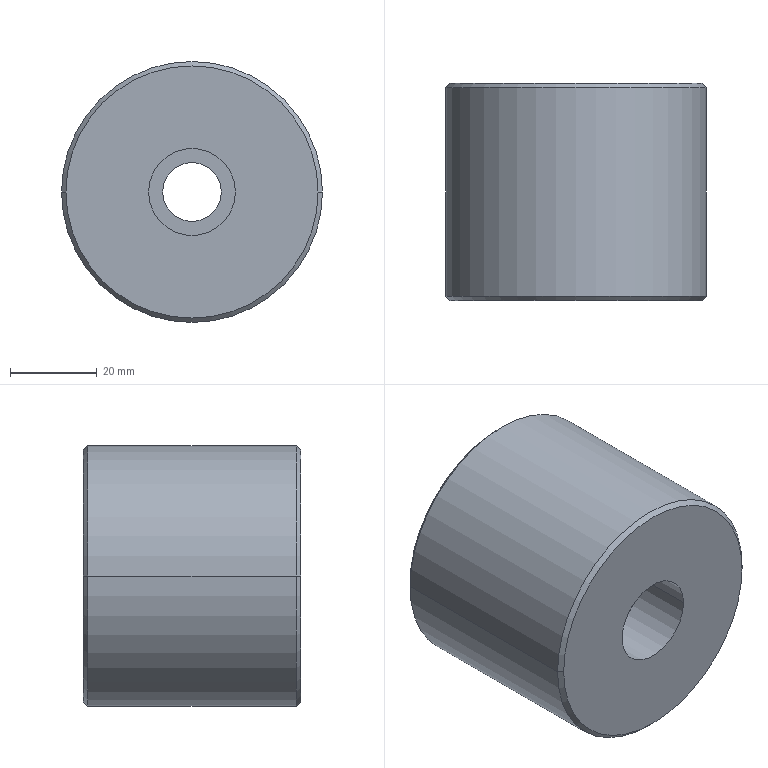Part | Creo | 1 solid | 13 faces | box 60 x 50 x 60 mm | volume 131634 mm3 | cylinder 6 | cone 4 | plane 3 | commonest cylinder face diameters 13.5 x2 20 x2 60 x2
STEP:
#1=CARTESIAN_POINT('',(0.,0.,0.));
#2=DIRECTION('',(0.,0.,1.));
#3=DIRECTION('',(1.,0.,0.));
#4=AXIS2_PLACEMENT_3D('',#1,#2,#3);
#5=CARTESIAN_POINT('',(-195.,-251.,-52.5));
#6=VERTEX_POINT('',#5);
#7=CARTESIAN_POINT('',(-135.,-251.,-52.5));
#8=VERTEX_POINT('',#7);
#9=CARTESIAN_POINT('',(-165.,-251.,-52.5));
#10=DIRECTION('',(0.,1.,0.));
#11=DIRECTION('',(-1.,0.,0.));
#12=AXIS2_PLACEMENT_3D('',#9,#10,#11);
#13=CIRCLE('',#12,30.);
#14=EDGE_CURVE('',#6,#8,#13,.T.);
#15=ORIENTED_EDGE('',*,*,#14,.T.);
#16=CARTESIAN_POINT('',(-135.,-299.,-52.5));
#17=VERTEX_POINT('',#16);
#18=CARTESIAN_POINT('',(-135.,-299.,-52.5));
#19=DIRECTION('',(0.,1.,0.));
#20=VECTOR('',#19,48.);
#21=LINE('',#18,#20);
#22=EDGE_CURVE('',#17,#8,#21,.T.);
#23=ORIENTED_EDGE('',*,*,#22,.F.);
#24=CARTESIAN_POINT('',(-195.,-299.,-52.5));
#25=VERTEX_POINT('',#24);
#26=CARTESIAN_POINT('',(-165.,-299.,-52.5));
#27=DIRECTION('',(0.,-1.,0.));
#28=DIRECTION('',(1.,0.,0.));
#29=AXIS2_PLACEMENT_3D('',#26,#27,#28);
#30=CIRCLE('',#29,30.);
#31=EDGE_CURVE('',#17,#25,#30,.T.);
#32=ORIENTED_EDGE('',*,*,#31,.T.);
#33=CARTESIAN_POINT('',(-195.,-299.,-52.5));
#34=DIRECTION('',(0.,1.,0.));
#35=VECTOR('',#34,48.);
#36=LINE('',#33,#35);
#37=EDGE_CURVE('',#25,#6,#36,.T.);
#38=ORIENTED_EDGE('',*,*,#37,.T.);
#39=EDGE_LOOP('',(#15,#23,#32,#38));
#40=FACE_OUTER_BOUND('',#39,.F.);
#41=CARTESIAN_POINT('',(-165.,-300.,-52.5));
#42=DIRECTION('',(0.,1.,0.));
#43=DIRECTION('',(-1.,0.,0.));
#44=AXIS2_PLACEMENT_3D('',#41,#42,#43);
#45=CYLINDRICAL_SURFACE('',#44,30.);
#46=ADVANCED_FACE('',(#40),#45,.T.);
#47=CARTESIAN_POINT('',(-194.,-250.,-52.5));
#48=VERTEX_POINT('',#47);
#49=CARTESIAN_POINT('',(-136.,-250.,-52.5));
#50=VERTEX_POINT('',#49);
#51=CARTESIAN_POINT('',(-165.,-250.,-52.5));
#52=DIRECTION('',(0.,1.,0.));
#53=DIRECTION('',(-1.,0.,0.));
#54=AXIS2_PLACEMENT_3D('',#51,#52,#53);
#55=CIRCLE('',#54,29.);
#56=EDGE_CURVE('',#48,#50,#55,.T.);
#57=ORIENTED_EDGE('',*,*,#56,.T.);
#58=CARTESIAN_POINT('',(-136.,-250.,-52.5));
#59=DIRECTION('',(0.7071,-0.7071,0.));
#60=VECTOR('',#59,1.414);
#61=LINE('',#58,#60);
#62=EDGE_CURVE('',#50,#8,#61,.T.);
#63=ORIENTED_EDGE('',*,*,#62,.T.);
#64=ORIENTED_EDGE('',*,*,#14,.F.);
#65=CARTESIAN_POINT('',(-194.,-250.,-52.5));
#66=DIRECTION('',(-0.7071,-0.7071,0.));
#67=VECTOR('',#66,1.414);
#68=LINE('',#65,#67);
#69=EDGE_CURVE('',#48,#6,#68,.T.);
#70=ORIENTED_EDGE('',*,*,#69,.F.);
#71=EDGE_LOOP('',(#57,#63,#64,#70));
#72=FACE_OUTER_BOUND('',#71,.F.);
#73=CARTESIAN_POINT('',(-165.,-250.5,-52.5));
#74=DIRECTION('',(0.,-1.,0.));
#75=DIRECTION('',(1.,0.,0.));
#76=AXIS2_PLACEMENT_3D('',#73,#74,#75);
#77=CONICAL_SURFACE('',#76,29.5,45.);
#78=ADVANCED_FACE('',(#72),#77,.T.);
#79=CARTESIAN_POINT('',(-165.,-250.,-52.5));
#80=DIRECTION('',(0.,1.,0.));
#81=DIRECTION('',(1.,0.,0.));
#82=AXIS2_PLACEMENT_3D('',#79,#80,#81);
#83=CIRCLE('',#82,29.);
#84=EDGE_CURVE('',#50,#48,#83,.T.);
#85=ORIENTED_EDGE('',*,*,#84,.F.);
#86=ORIENTED_EDGE('',*,*,#56,.F.);
#87=EDGE_LOOP('',(#85,#86));
#88=FACE_OUTER_BOUND('',#87,.F.);
#89=CARTESIAN_POINT('',(-171.75,-250.,-52.5));
#90=VERTEX_POINT('',#89);
#91=CARTESIAN_POINT('',(-158.25,-250.,-52.5));
#92=VERTEX_POINT('',#91);
#93=CARTESIAN_POINT('',(-165.,-250.,-52.5));
#94=DIRECTION('',(0.,-1.,0.));
#95=DIRECTION('',(-1.,0.,0.));
#96=AXIS2_PLACEMENT_3D('',#93,#94,#95);
#97=CIRCLE('',#96,6.75);
#98=EDGE_CURVE('',#90,#92,#97,.T.);
#99=ORIENTED_EDGE('',*,*,#98,.F.);
#100=CARTESIAN_POINT('',(-165.,-250.,-52.5));
#101=DIRECTION('',(0.,-1.,0.));
#102=DIRECTION('',(1.,0.,0.));
#103=AXIS2_PLACEMENT_3D('',#100,#101,#102);
#104=CIRCLE('',#103,6.75);
#105=EDGE_CURVE('',#92,#90,#104,.T.);
#106=ORIENTED_EDGE('',*,*,#105,.F.);
#107=EDGE_LOOP('',(#99,#106));
#108=FACE_BOUND('',#107,.F.);
#109=CARTESIAN_POINT('',(-165.,-250.,-52.5));
#110=DIRECTION('',(0.,-1.,0.));
#111=DIRECTION('',(1.,0.,0.));
#112=AXIS2_PLACEMENT_3D('',#109,#110,#111);
#113=PLANE('',#112);
#114=ADVANCED_FACE('',(#88,#108),#113,.F.);
#115=ORIENTED_EDGE('',*,*,#98,.T.);
#116=CARTESIAN_POINT('',(-158.25,-286.,-52.5));
#117=VERTEX_POINT('',#116);
#118=CARTESIAN_POINT('',(-158.25,-250.,-52.5));
#119=DIRECTION('',(0.,-1.,0.));
#120=VECTOR('',#119,36.);
#121=LINE('',#118,#120);
#122=EDGE_CURVE('',#92,#117,#121,.T.);
#123=ORIENTED_EDGE('',*,*,#122,.T.);
#124=CARTESIAN_POINT('',(-171.75,-286.,-52.5));
#125=VERTEX_POINT('',#124);
#126=CARTESIAN_POINT('',(-165.,-286.,-52.5));
#127=DIRECTION('',(0.,1.,0.));
#128=DIRECTION('',(1.,0.,0.));
#129=AXIS2_PLACEMENT_3D('',#126,#127,#128);
#130=CIRCLE('',#129,6.75);
#131=EDGE_CURVE('',#117,#125,#130,.T.);
#132=ORIENTED_EDGE('',*,*,#131,.T.);
#133=CARTESIAN_POINT('',(-171.75,-250.,-52.5));
#134=DIRECTION('',(0.,-1.,0.));
#135=VECTOR('',#134,36.);
#136=LINE('',#133,#135);
#137=EDGE_CURVE('',#90,#125,#136,.T.);
#138=ORIENTED_EDGE('',*,*,#137,.F.);
#139=EDGE_LOOP('',(#115,#123,#132,#138));
#140=FACE_OUTER_BOUND('',#139,.F.);
#141=CARTESIAN_POINT('',(-165.,-300.,-52.5));
#142=DIRECTION('',(0.,-1.,0.));
#143=DIRECTION('',(-1.,0.,0.));
#144=AXIS2_PLACEMENT_3D('',#141,#142,#143);
#145=CYLINDRICAL_SURFACE('',#144,6.75);
#146=ADVANCED_FACE('',(#140),#145,.F.);
#147=ORIENTED_EDGE('',*,*,#105,.T.);
#148=ORIENTED_EDGE('',*,*,#137,.T.);
#149=CARTESIAN_POINT('',(-165.,-286.,-52.5));
#150=DIRECTION('',(0.,1.,0.));
#151=DIRECTION('',(-1.,0.,0.));
#152=AXIS2_PLACEMENT_3D('',#149,#150,#151);
#153=CIRCLE('',#152,6.75);
#154=EDGE_CURVE('',#125,#117,#153,.T.);
#155=ORIENTED_EDGE('',*,*,#154,.T.);
#156=ORIENTED_EDGE('',*,*,#122,.F.);
#157=EDGE_LOOP('',(#147,#148,#155,#156));
#158=FACE_OUTER_BOUND('',#157,.F.);
#159=CARTESIAN_POINT('',(-165.,-300.,-52.5));
#160=DIRECTION('',(0.,-1.,0.));
#161=DIRECTION('',(-1.,0.,0.));
#162=AXIS2_PLACEMENT_3D('',#159,#160,#161);
#163=CYLINDRICAL_SURFACE('',#162,6.75);
#164=ADVANCED_FACE('',(#158),#163,.F.);
#165=CARTESIAN_POINT('',(-175.,-286.,-52.5));
#166=VERTEX_POINT('',#165);
#167=CARTESIAN_POINT('',(-155.,-286.,-52.5));
#168=VERTEX_POINT('',#167);
#169=CARTESIAN_POINT('',(-165.,-286.,-52.5));
#170=DIRECTION('',(0.,-1.,0.));
#171=DIRECTION('',(-1.,0.,0.));
#172=AXIS2_PLACEMENT_3D('',#169,#170,#171);
#173=CIRCLE('',#172,10.);
#174=EDGE_CURVE('',#166,#168,#173,.T.);
#175=ORIENTED_EDGE('',*,*,#174,.F.);
#176=CARTESIAN_POINT('',(-165.,-286.,-52.5));
#177=DIRECTION('',(0.,-1.,0.));
#178=DIRECTION('',(1.,0.,0.));
#179=AXIS2_PLACEMENT_3D('',#176,#177,#178);
#180=CIRCLE('',#179,10.);
#181=EDGE_CURVE('',#168,#166,#180,.T.);
#182=ORIENTED_EDGE('',*,*,#181,.F.);
#183=EDGE_LOOP('',(#175,#182));
#184=FACE_OUTER_BOUND('',#183,.F.);
#185=ORIENTED_EDGE('',*,*,#154,.F.);
#186=ORIENTED_EDGE('',*,*,#131,.F.);
#187=EDGE_LOOP('',(#185,#186));
#188=FACE_BOUND('',#187,.F.);
#189=CARTESIAN_POINT('',(-165.,-286.,-62.5));
#190=DIRECTION('',(0.,1.,0.));
#191=DIRECTION('',(1.,0.,0.));
#192=AXIS2_PLACEMENT_3D('',#189,#190,#191);
#193=PLANE('',#192);
#194=ADVANCED_FACE('',(#184,#188),#193,.F.);
#195=ORIENTED_EDGE('',*,*,#174,.T.);
#196=CARTESIAN_POINT('',(-155.,-300.,-52.5));
#197=VERTEX_POINT('',#196);
#198=CARTESIAN_POINT('',(-155.,-286.,-52.5));
#199=DIRECTION('',(0.,-1.,0.));
#200=VECTOR('',#199,14.);
#201=LINE('',#198,#200);
#202=EDGE_CURVE('',#168,#197,#201,.T.);
#203=ORIENTED_EDGE('',*,*,#202,.T.);
#204=CARTESIAN_POINT('',(-175.,-300.,-52.5));
#205=VERTEX_POINT('',#204);
#206=CARTESIAN_POINT('',(-165.,-300.,-52.5));
#207=DIRECTION('',(0.,1.,0.));
#208=DIRECTION('',(1.,0.,0.));
#209=AXIS2_PLACEMENT_3D('',#206,#207,#208);
#210=CIRCLE('',#209,10.);
#211=EDGE_CURVE('',#197,#205,#210,.T.);
#212=ORIENTED_EDGE('',*,*,#211,.T.);
#213=CARTESIAN_POINT('',(-175.,-286.,-52.5));
#214=DIRECTION('',(0.,-1.,0.));
#215=VECTOR('',#214,14.);
#216=LINE('',#213,#215);
#217=EDGE_CURVE('',#166,#205,#216,.T.);
#218=ORIENTED_EDGE('',*,*,#217,.F.);
#219=EDGE_LOOP('',(#195,#203,#212,#218));
#220=FACE_OUTER_BOUND('',#219,.F.);
#221=CARTESIAN_POINT('',(-165.,-300.,-52.5));
#222=DIRECTION('',(0.,-1.,0.));
#223=DIRECTION('',(-1.,0.,0.));
#224=AXIS2_PLACEMENT_3D('',#221,#222,#223);
#225=CYLINDRICAL_SURFACE('',#224,10.);
#226=ADVANCED_FACE('',(#220),#225,.F.);
#227=ORIENTED_EDGE('',*,*,#181,.T.);
#228=ORIENTED_EDGE('',*,*,#217,.T.);
#229=CARTESIAN_POINT('',(-165.,-300.,-52.5));
#230=DIRECTION('',(0.,1.,0.));
#231=DIRECTION('',(-1.,0.,0.));
#232=AXIS2_PLACEMENT_3D('',#229,#230,#231);
#233=CIRCLE('',#232,10.);
#234=EDGE_CURVE('',#205,#197,#233,.T.);
#235=ORIENTED_EDGE('',*,*,#234,.T.);
#236=ORIENTED_EDGE('',*,*,#202,.F.);
#237=EDGE_LOOP('',(#227,#228,#235,#236));
#238=FACE_OUTER_BOUND('',#237,.F.);
#239=CARTESIAN_POINT('',(-165.,-300.,-52.5));
#240=DIRECTION('',(0.,-1.,0.));
#241=DIRECTION('',(-1.,0.,0.));
#242=AXIS2_PLACEMENT_3D('',#239,#240,#241);
#243=CYLINDRICAL_SURFACE('',#242,10.);
#244=ADVANCED_FACE('',(#238),#243,.F.);
#245=CARTESIAN_POINT('',(-136.,-300.,-52.5));
#246=VERTEX_POINT('',#245);
#247=CARTESIAN_POINT('',(-194.,-300.,-52.5));
#248=VERTEX_POINT('',#247);
#249=CARTESIAN_POINT('',(-165.,-300.,-52.5));
#250=DIRECTION('',(0.,-1.,0.));
#251=DIRECTION('',(1.,0.,0.));
#252=AXIS2_PLACEMENT_3D('',#249,#250,#251);
#253=CIRCLE('',#252,29.);
#254=EDGE_CURVE('',#246,#248,#253,.T.);
#255=ORIENTED_EDGE('',*,*,#254,.F.);
#256=CARTESIAN_POINT('',(-165.,-300.,-52.5));
#257=DIRECTION('',(0.,-1.,0.));
#258=DIRECTION('',(-1.,0.,0.));
#259=AXIS2_PLACEMENT_3D('',#256,#257,#258);
#260=CIRCLE('',#259,29.);
#261=EDGE_CURVE('',#248,#246,#260,.T.);
#262=ORIENTED_EDGE('',*,*,#261,.F.);
#263=EDGE_LOOP('',(#255,#262));
#264=FACE_OUTER_BOUND('',#263,.F.);
#265=ORIENTED_EDGE('',*,*,#234,.F.);
#266=ORIENTED_EDGE('',*,*,#211,.F.);
#267=EDGE_LOOP('',(#265,#266));
#268=FACE_BOUND('',#267,.F.);
#269=CARTESIAN_POINT('',(-165.,-300.,-52.5));
#270=DIRECTION('',(0.,-1.,0.));
#271=DIRECTION('',(1.,0.,0.));
#272=AXIS2_PLACEMENT_3D('',#269,#270,#271);
#273=PLANE('',#272);
#274=ADVANCED_FACE('',(#264,#268),#273,.T.);
#275=ORIENTED_EDGE('',*,*,#31,.F.);
#276=CARTESIAN_POINT('',(-136.,-300.,-52.5));
#277=DIRECTION('',(0.7071,0.7071,0.));
#278=VECTOR('',#277,1.414);
#279=LINE('',#276,#278);
#280=EDGE_CURVE('',#246,#17,#279,.T.);
#281=ORIENTED_EDGE('',*,*,#280,.F.);
#282=ORIENTED_EDGE('',*,*,#254,.T.);
#283=CARTESIAN_POINT('',(-194.,-300.,-52.5));
#284=DIRECTION('',(-0.7071,0.7071,0.));
#285=VECTOR('',#284,1.414);
#286=LINE('',#283,#285);
#287=EDGE_CURVE('',#248,#25,#286,.T.);
#288=ORIENTED_EDGE('',*,*,#287,.T.);
#289=EDGE_LOOP('',(#275,#281,#282,#288));
#290=FACE_OUTER_BOUND('',#289,.F.);
#291=CARTESIAN_POINT('',(-165.,-299.5,-52.5));
#292=DIRECTION('',(0.,1.,0.));
#293=DIRECTION('',(-1.,0.,0.));
#294=AXIS2_PLACEMENT_3D('',#291,#292,#293);
#295=CONICAL_SURFACE('',#294,29.5,45.);
#296=ADVANCED_FACE('',(#290),#295,.T.);
#297=CARTESIAN_POINT('',(-165.,-299.,-52.5));
#298=DIRECTION('',(0.,-1.,0.));
#299=DIRECTION('',(-1.,0.,0.));
#300=AXIS2_PLACEMENT_3D('',#297,#298,#299);
#301=CIRCLE('',#300,30.);
#302=EDGE_CURVE('',#25,#17,#301,.T.);
#303=ORIENTED_EDGE('',*,*,#302,.F.);
#304=ORIENTED_EDGE('',*,*,#287,.F.);
#305=ORIENTED_EDGE('',*,*,#261,.T.);
#306=ORIENTED_EDGE('',*,*,#280,.T.);
#307=EDGE_LOOP('',(#303,#304,#305,#306));
#308=FACE_OUTER_BOUND('',#307,.F.);
#309=CARTESIAN_POINT('',(-165.,-299.5,-52.5));
#310=DIRECTION('',(0.,1.,0.));
#311=DIRECTION('',(-1.,0.,0.));
#312=AXIS2_PLACEMENT_3D('',#309,#310,#311);
#313=CONICAL_SURFACE('',#312,29.5,45.);
#314=ADVANCED_FACE('',(#308),#313,.T.);
#315=CARTESIAN_POINT('',(-165.,-251.,-52.5));
#316=DIRECTION('',(0.,1.,0.));
#317=DIRECTION('',(1.,0.,0.));
#318=AXIS2_PLACEMENT_3D('',#315,#316,#317);
#319=CIRCLE('',#318,30.);
#320=EDGE_CURVE('',#8,#6,#319,.T.);
#321=ORIENTED_EDGE('',*,*,#320,.T.);
#322=ORIENTED_EDGE('',*,*,#37,.F.);
#323=ORIENTED_EDGE('',*,*,#302,.T.);
#324=ORIENTED_EDGE('',*,*,#22,.T.);
#325=EDGE_LOOP('',(#321,#322,#323,#324));
#326=FACE_OUTER_BOUND('',#325,.F.);
#327=CARTESIAN_POINT('',(-165.,-300.,-52.5));
#328=DIRECTION('',(0.,1.,0.));
#329=DIRECTION('',(-1.,0.,0.));
#330=AXIS2_PLACEMENT_3D('',#327,#328,#329);
#331=CYLINDRICAL_SURFACE('',#330,30.);
#332=ADVANCED_FACE('',(#326),#331,.T.);
#333=ORIENTED_EDGE('',*,*,#84,.T.);
#334=ORIENTED_EDGE('',*,*,#69,.T.);
#335=ORIENTED_EDGE('',*,*,#320,.F.);
#336=ORIENTED_EDGE('',*,*,#62,.F.);
#337=EDGE_LOOP('',(#333,#334,#335,#336));
#338=FACE_OUTER_BOUND('',#337,.F.);
#339=CARTESIAN_POINT('',(-165.,-250.5,-52.5));
#340=DIRECTION('',(0.,-1.,0.));
#341=DIRECTION('',(1.,0.,0.));
#342=AXIS2_PLACEMENT_3D('',#339,#340,#341);
#343=CONICAL_SURFACE('',#342,29.5,45.);
#344=ADVANCED_FACE('',(#338),#343,.T.);
#345=CLOSED_SHELL('',(#46,#78,#114,#146,#164,#194,#226,#244,#274,#296,#314,#332,#344));
#346=MANIFOLD_SOLID_BREP('',#345);
#347=(LENGTH_UNIT()NAMED_UNIT(*)SI_UNIT(.MILLI.,.METRE.));
#348=UNCERTAINTY_MEASURE_WITH_UNIT(LENGTH_MEASURE(0.009848),#347,'','');
#349=(NAMED_UNIT(*)PLANE_ANGLE_UNIT()SI_UNIT($,.RADIAN.));
#350=PLANE_ANGLE_MEASURE_WITH_UNIT(PLANE_ANGLE_MEASURE(0.01745),#349);
#351=(CONVERSION_BASED_UNIT('DEGREE',#350)NAMED_UNIT(*)PLANE_ANGLE_UNIT());
#352=(NAMED_UNIT(*)SI_UNIT($,.STERADIAN.)SOLID_ANGLE_UNIT());
#353=(GEOMETRIC_REPRESENTATION_CONTEXT(3)GLOBAL_UNCERTAINTY_ASSIGNED_CONTEXT((#348))GLOBAL_UNIT_ASSIGNED_CONTEXT((#347,#351,#352))REPRESENTATION_CONTEXT('',''));
#354=ADVANCED_BREP_SHAPE_REPRESENTATION('',(#4,#346),#353);